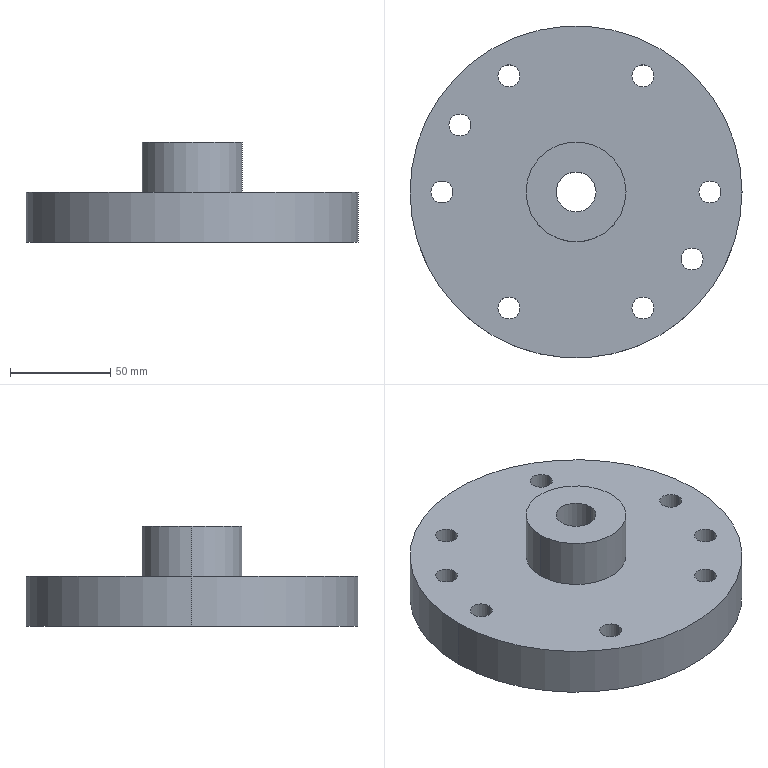Part | SolidWorks | features ICE 5, Chamfer 1, Extrusion 1 | 1 solid | 34 faces | box 166 x 166 x 50 mm | volume 495390 mm3 | cylinder 26 | plane 6 | cone 2 | commonest cylinder face diameters 11 x16 18 x4 20 x2 50 x2 166 x2
STEP:
#1=CARTESIAN_POINT('',(42.5,-58.024,12.));
#2=VERTEX_POINT('',#1);
#3=CARTESIAN_POINT('',(24.5,-58.024,12.));
#4=VERTEX_POINT('',#3);
#5=CARTESIAN_POINT('',(33.5,-58.024,12.));
#6=DIRECTION('',(0.,0.,-1.));
#7=DIRECTION('',(-1.,0.,0.));
#8=AXIS2_PLACEMENT_3D('',#5,#6,#7);
#9=CIRCLE('',#8,9.);
#10=EDGE_CURVE('',#2,#4,#9,.T.);
#11=ORIENTED_EDGE('',*,*,#10,.F.);
#12=CARTESIAN_POINT('',(42.5,-58.024,0.));
#13=VERTEX_POINT('',#12);
#14=CARTESIAN_POINT('',(42.5,-58.024,12.));
#15=DIRECTION('',(0.,0.,-1.));
#16=VECTOR('',#15,1000.);
#17=LINE('',#14,#16);
#18=EDGE_CURVE('',#2,#13,#17,.T.);
#19=ORIENTED_EDGE('',*,*,#18,.T.);
#20=CARTESIAN_POINT('',(24.5,-58.024,0.));
#21=VERTEX_POINT('',#20);
#22=CARTESIAN_POINT('',(33.5,-58.024,0.));
#23=DIRECTION('',(0.,0.,-1.));
#24=DIRECTION('',(-1.,0.,0.));
#25=AXIS2_PLACEMENT_3D('',#22,#23,#24);
#26=CIRCLE('',#25,9.);
#27=EDGE_CURVE('',#13,#21,#26,.T.);
#28=ORIENTED_EDGE('',*,*,#27,.T.);
#29=CARTESIAN_POINT('',(24.5,-58.024,12.));
#30=DIRECTION('',(0.,0.,-1.));
#31=VECTOR('',#30,1000.);
#32=LINE('',#29,#31);
#33=EDGE_CURVE('',#4,#21,#32,.T.);
#34=ORIENTED_EDGE('',*,*,#33,.F.);
#35=EDGE_LOOP('',(#11,#19,#28,#34));
#36=FACE_OUTER_BOUND('',#35,.T.);
#37=CARTESIAN_POINT('',(33.5,-58.024,12.));
#38=DIRECTION('',(0.,0.,-1.));
#39=DIRECTION('',(-1.,0.,0.));
#40=AXIS2_PLACEMENT_3D('',#37,#38,#39);
#41=CYLINDRICAL_SURFACE('',#40,9.);
#42=ADVANCED_FACE('',(#36),#41,.F.);
#43=CARTESIAN_POINT('',(-24.5,58.024,12.));
#44=VERTEX_POINT('',#43);
#45=CARTESIAN_POINT('',(-42.5,58.024,12.));
#46=VERTEX_POINT('',#45);
#47=CARTESIAN_POINT('',(-33.5,58.024,12.));
#48=DIRECTION('',(0.,0.,-1.));
#49=DIRECTION('',(-1.,0.,0.));
#50=AXIS2_PLACEMENT_3D('',#47,#48,#49);
#51=CIRCLE('',#50,9.);
#52=EDGE_CURVE('',#44,#46,#51,.T.);
#53=ORIENTED_EDGE('',*,*,#52,.F.);
#54=CARTESIAN_POINT('',(-24.5,58.024,0.));
#55=VERTEX_POINT('',#54);
#56=CARTESIAN_POINT('',(-24.5,58.024,12.));
#57=DIRECTION('',(0.,0.,-1.));
#58=VECTOR('',#57,1000.);
#59=LINE('',#56,#58);
#60=EDGE_CURVE('',#44,#55,#59,.T.);
#61=ORIENTED_EDGE('',*,*,#60,.T.);
#62=CARTESIAN_POINT('',(-42.5,58.024,0.));
#63=VERTEX_POINT('',#62);
#64=CARTESIAN_POINT('',(-33.5,58.024,0.));
#65=DIRECTION('',(0.,0.,-1.));
#66=DIRECTION('',(-1.,0.,0.));
#67=AXIS2_PLACEMENT_3D('',#64,#65,#66);
#68=CIRCLE('',#67,9.);
#69=EDGE_CURVE('',#55,#63,#68,.T.);
#70=ORIENTED_EDGE('',*,*,#69,.T.);
#71=CARTESIAN_POINT('',(-42.5,58.024,12.));
#72=DIRECTION('',(0.,0.,-1.));
#73=VECTOR('',#72,1000.);
#74=LINE('',#71,#73);
#75=EDGE_CURVE('',#46,#63,#74,.T.);
#76=ORIENTED_EDGE('',*,*,#75,.F.);
#77=EDGE_LOOP('',(#53,#61,#70,#76));
#78=FACE_OUTER_BOUND('',#77,.T.);
#79=CARTESIAN_POINT('',(-33.5,58.024,12.));
#80=DIRECTION('',(0.,0.,-1.));
#81=DIRECTION('',(-1.,0.,0.));
#82=AXIS2_PLACEMENT_3D('',#79,#80,#81);
#83=CYLINDRICAL_SURFACE('',#82,9.);
#84=ADVANCED_FACE('',(#78),#83,.F.);
#85=CARTESIAN_POINT('',(10.,0.,50.));
#86=VERTEX_POINT('',#85);
#87=CARTESIAN_POINT('',(-10.,0.,50.));
#88=VERTEX_POINT('',#87);
#89=CARTESIAN_POINT('',(0.,0.,50.));
#90=DIRECTION('',(0.,0.,-1.));
#91=DIRECTION('',(-1.,0.,0.));
#92=AXIS2_PLACEMENT_3D('',#89,#90,#91);
#93=CIRCLE('',#92,10.);
#94=EDGE_CURVE('',#86,#88,#93,.T.);
#95=ORIENTED_EDGE('',*,*,#94,.F.);
#96=CARTESIAN_POINT('',(10.,0.,7.));
#97=VERTEX_POINT('',#96);
#98=CARTESIAN_POINT('',(10.,0.,50.));
#99=DIRECTION('',(0.,0.,-1.));
#100=VECTOR('',#99,1000.);
#101=LINE('',#98,#100);
#102=EDGE_CURVE('',#86,#97,#101,.T.);
#103=ORIENTED_EDGE('',*,*,#102,.T.);
#104=CARTESIAN_POINT('',(-10.,0.,7.));
#105=VERTEX_POINT('',#104);
#106=CARTESIAN_POINT('',(0.,0.,7.));
#107=DIRECTION('',(0.,0.,-1.));
#108=DIRECTION('',(-1.,0.,0.));
#109=AXIS2_PLACEMENT_3D('',#106,#107,#108);
#110=CIRCLE('',#109,10.);
#111=EDGE_CURVE('',#97,#105,#110,.T.);
#112=ORIENTED_EDGE('',*,*,#111,.T.);
#113=CARTESIAN_POINT('',(-10.,0.,50.));
#114=DIRECTION('',(0.,0.,-1.));
#115=VECTOR('',#114,1000.);
#116=LINE('',#113,#115);
#117=EDGE_CURVE('',#88,#105,#116,.T.);
#118=ORIENTED_EDGE('',*,*,#117,.F.);
#119=EDGE_LOOP('',(#95,#103,#112,#118));
#120=FACE_OUTER_BOUND('',#119,.T.);
#121=CARTESIAN_POINT('',(0.,0.,50.));
#122=DIRECTION('',(0.,0.,-1.));
#123=DIRECTION('',(-1.,0.,0.));
#124=AXIS2_PLACEMENT_3D('',#121,#122,#123);
#125=CYLINDRICAL_SURFACE('',#124,10.);
#126=ADVANCED_FACE('',(#120),#125,.F.);
#127=CARTESIAN_POINT('',(-63.524,33.5,25.));
#128=VERTEX_POINT('',#127);
#129=CARTESIAN_POINT('',(-52.524,33.5,25.));
#130=VERTEX_POINT('',#129);
#131=CARTESIAN_POINT('',(-58.024,33.5,25.));
#132=DIRECTION('',(0.,0.,1.));
#133=DIRECTION('',(1.,0.,0.));
#134=AXIS2_PLACEMENT_3D('',#131,#132,#133);
#135=CIRCLE('',#134,5.5);
#136=EDGE_CURVE('',#128,#130,#135,.T.);
#137=ORIENTED_EDGE('',*,*,#136,.T.);
#138=CARTESIAN_POINT('',(-52.524,33.5,0.));
#139=VERTEX_POINT('',#138);
#140=CARTESIAN_POINT('',(-52.524,33.5,50.));
#141=DIRECTION('',(0.,0.,-1.));
#142=VECTOR('',#141,1000.);
#143=LINE('',#140,#142);
#144=EDGE_CURVE('',#130,#139,#143,.T.);
#145=ORIENTED_EDGE('',*,*,#144,.T.);
#146=CARTESIAN_POINT('',(-63.524,33.5,0.));
#147=VERTEX_POINT('',#146);
#148=CARTESIAN_POINT('',(-58.024,33.5,0.));
#149=DIRECTION('',(0.,0.,-1.));
#150=DIRECTION('',(-1.,0.,0.));
#151=AXIS2_PLACEMENT_3D('',#148,#149,#150);
#152=CIRCLE('',#151,5.5);
#153=EDGE_CURVE('',#139,#147,#152,.T.);
#154=ORIENTED_EDGE('',*,*,#153,.T.);
#155=CARTESIAN_POINT('',(-63.524,33.5,50.));
#156=DIRECTION('',(0.,0.,-1.));
#157=VECTOR('',#156,1000.);
#158=LINE('',#155,#157);
#159=EDGE_CURVE('',#128,#147,#158,.T.);
#160=ORIENTED_EDGE('',*,*,#159,.F.);
#161=EDGE_LOOP('',(#137,#145,#154,#160));
#162=FACE_OUTER_BOUND('',#161,.T.);
#163=CARTESIAN_POINT('',(-58.024,33.5,50.));
#164=DIRECTION('',(0.,0.,-1.));
#165=DIRECTION('',(-1.,0.,0.));
#166=AXIS2_PLACEMENT_3D('',#163,#164,#165);
#167=CYLINDRICAL_SURFACE('',#166,5.5);
#168=ADVANCED_FACE('',(#162),#167,.F.);
#169=CARTESIAN_POINT('',(-39.,-58.024,25.));
#170=VERTEX_POINT('',#169);
#171=CARTESIAN_POINT('',(-28.,-58.024,25.));
#172=VERTEX_POINT('',#171);
#173=CARTESIAN_POINT('',(-33.5,-58.024,25.));
#174=DIRECTION('',(0.,0.,1.));
#175=DIRECTION('',(1.,0.,0.));
#176=AXIS2_PLACEMENT_3D('',#173,#174,#175);
#177=CIRCLE('',#176,5.5);
#178=EDGE_CURVE('',#170,#172,#177,.T.);
#179=ORIENTED_EDGE('',*,*,#178,.T.);
#180=CARTESIAN_POINT('',(-28.,-58.024,0.));
#181=VERTEX_POINT('',#180);
#182=CARTESIAN_POINT('',(-28.,-58.024,50.));
#183=DIRECTION('',(0.,0.,-1.));
#184=VECTOR('',#183,1000.);
#185=LINE('',#182,#184);
#186=EDGE_CURVE('',#172,#181,#185,.T.);
#187=ORIENTED_EDGE('',*,*,#186,.T.);
#188=CARTESIAN_POINT('',(-39.,-58.024,0.));
#189=VERTEX_POINT('',#188);
#190=CARTESIAN_POINT('',(-33.5,-58.024,0.));
#191=DIRECTION('',(0.,0.,-1.));
#192=DIRECTION('',(-1.,0.,0.));
#193=AXIS2_PLACEMENT_3D('',#190,#191,#192);
#194=CIRCLE('',#193,5.5);
#195=EDGE_CURVE('',#181,#189,#194,.T.);
#196=ORIENTED_EDGE('',*,*,#195,.T.);
#197=CARTESIAN_POINT('',(-39.,-58.024,50.));
#198=DIRECTION('',(0.,0.,-1.));
#199=VECTOR('',#198,1000.);
#200=LINE('',#197,#199);
#201=EDGE_CURVE('',#170,#189,#200,.T.);
#202=ORIENTED_EDGE('',*,*,#201,.F.);
#203=EDGE_LOOP('',(#179,#187,#196,#202));
#204=FACE_OUTER_BOUND('',#203,.T.);
#205=CARTESIAN_POINT('',(-33.5,-58.024,50.));
#206=DIRECTION('',(0.,0.,-1.));
#207=DIRECTION('',(-1.,0.,0.));
#208=AXIS2_PLACEMENT_3D('',#205,#206,#207);
#209=CYLINDRICAL_SURFACE('',#208,5.5);
#210=ADVANCED_FACE('',(#204),#209,.F.);
#211=CARTESIAN_POINT('',(52.524,-33.5,25.));
#212=VERTEX_POINT('',#211);
#213=CARTESIAN_POINT('',(63.524,-33.5,25.));
#214=VERTEX_POINT('',#213);
#215=CARTESIAN_POINT('',(58.024,-33.5,25.));
#216=DIRECTION('',(0.,0.,1.));
#217=DIRECTION('',(1.,0.,0.));
#218=AXIS2_PLACEMENT_3D('',#215,#216,#217);
#219=CIRCLE('',#218,5.5);
#220=EDGE_CURVE('',#212,#214,#219,.T.);
#221=ORIENTED_EDGE('',*,*,#220,.T.);
#222=CARTESIAN_POINT('',(63.524,-33.5,0.));
#223=VERTEX_POINT('',#222);
#224=CARTESIAN_POINT('',(63.524,-33.5,50.));
#225=DIRECTION('',(0.,0.,-1.));
#226=VECTOR('',#225,1000.);
#227=LINE('',#224,#226);
#228=EDGE_CURVE('',#214,#223,#227,.T.);
#229=ORIENTED_EDGE('',*,*,#228,.T.);
#230=CARTESIAN_POINT('',(52.524,-33.5,0.));
#231=VERTEX_POINT('',#230);
#232=CARTESIAN_POINT('',(58.024,-33.5,0.));
#233=DIRECTION('',(0.,0.,-1.));
#234=DIRECTION('',(-1.,0.,0.));
#235=AXIS2_PLACEMENT_3D('',#232,#233,#234);
#236=CIRCLE('',#235,5.5);
#237=EDGE_CURVE('',#223,#231,#236,.T.);
#238=ORIENTED_EDGE('',*,*,#237,.T.);
#239=CARTESIAN_POINT('',(52.524,-33.5,50.));
#240=DIRECTION('',(0.,0.,-1.));
#241=VECTOR('',#240,1000.);
#242=LINE('',#239,#241);
#243=EDGE_CURVE('',#212,#231,#242,.T.);
#244=ORIENTED_EDGE('',*,*,#243,.F.);
#245=EDGE_LOOP('',(#221,#229,#238,#244));
#246=FACE_OUTER_BOUND('',#245,.T.);
#247=CARTESIAN_POINT('',(58.024,-33.5,50.));
#248=DIRECTION('',(0.,0.,-1.));
#249=DIRECTION('',(-1.,0.,0.));
#250=AXIS2_PLACEMENT_3D('',#247,#248,#249);
#251=CYLINDRICAL_SURFACE('',#250,5.5);
#252=ADVANCED_FACE('',(#246),#251,.F.);
#253=CARTESIAN_POINT('',(61.5,0.,25.));
#254=VERTEX_POINT('',#253);
#255=CARTESIAN_POINT('',(72.5,0.,25.));
#256=VERTEX_POINT('',#255);
#257=CARTESIAN_POINT('',(67.,0.,25.));
#258=DIRECTION('',(0.,0.,1.));
#259=DIRECTION('',(1.,0.,0.));
#260=AXIS2_PLACEMENT_3D('',#257,#258,#259);
#261=CIRCLE('',#260,5.5);
#262=EDGE_CURVE('',#254,#256,#261,.T.);
#263=ORIENTED_EDGE('',*,*,#262,.T.);
#264=CARTESIAN_POINT('',(72.5,0.,0.));
#265=VERTEX_POINT('',#264);
#266=CARTESIAN_POINT('',(72.5,0.,50.));
#267=DIRECTION('',(0.,0.,-1.));
#268=VECTOR('',#267,1000.);
#269=LINE('',#266,#268);
#270=EDGE_CURVE('',#256,#265,#269,.T.);
#271=ORIENTED_EDGE('',*,*,#270,.T.);
#272=CARTESIAN_POINT('',(61.5,0.,0.));
#273=VERTEX_POINT('',#272);
#274=CARTESIAN_POINT('',(67.,0.,0.));
#275=DIRECTION('',(0.,0.,-1.));
#276=DIRECTION('',(-1.,0.,0.));
#277=AXIS2_PLACEMENT_3D('',#274,#275,#276);
#278=CIRCLE('',#277,5.5);
#279=EDGE_CURVE('',#265,#273,#278,.T.);
#280=ORIENTED_EDGE('',*,*,#279,.T.);
#281=CARTESIAN_POINT('',(61.5,0.,50.));
#282=DIRECTION('',(0.,0.,-1.));
#283=VECTOR('',#282,1000.);
#284=LINE('',#281,#283);
#285=EDGE_CURVE('',#254,#273,#284,.T.);
#286=ORIENTED_EDGE('',*,*,#285,.F.);
#287=EDGE_LOOP('',(#263,#271,#280,#286));
#288=FACE_OUTER_BOUND('',#287,.T.);
#289=CARTESIAN_POINT('',(67.,0.,50.));
#290=DIRECTION('',(0.,0.,-1.));
#291=DIRECTION('',(-1.,0.,0.));
#292=AXIS2_PLACEMENT_3D('',#289,#290,#291);
#293=CYLINDRICAL_SURFACE('',#292,5.5);
#294=ADVANCED_FACE('',(#288),#293,.F.);
#295=CARTESIAN_POINT('',(28.,58.024,25.));
#296=VERTEX_POINT('',#295);
#297=CARTESIAN_POINT('',(39.,58.024,25.));
#298=VERTEX_POINT('',#297);
#299=CARTESIAN_POINT('',(33.5,58.024,25.));
#300=DIRECTION('',(0.,0.,1.));
#301=DIRECTION('',(1.,0.,0.));
#302=AXIS2_PLACEMENT_3D('',#299,#300,#301);
#303=CIRCLE('',#302,5.5);
#304=EDGE_CURVE('',#296,#298,#303,.T.);
#305=ORIENTED_EDGE('',*,*,#304,.T.);
#306=CARTESIAN_POINT('',(39.,58.024,0.));
#307=VERTEX_POINT('',#306);
#308=CARTESIAN_POINT('',(39.,58.024,50.));
#309=DIRECTION('',(0.,0.,-1.));
#310=VECTOR('',#309,1000.);
#311=LINE('',#308,#310);
#312=EDGE_CURVE('',#298,#307,#311,.T.);
#313=ORIENTED_EDGE('',*,*,#312,.T.);
#314=CARTESIAN_POINT('',(28.,58.024,0.));
#315=VERTEX_POINT('',#314);
#316=CARTESIAN_POINT('',(33.5,58.024,0.));
#317=DIRECTION('',(0.,0.,-1.));
#318=DIRECTION('',(-1.,0.,0.));
#319=AXIS2_PLACEMENT_3D('',#316,#317,#318);
#320=CIRCLE('',#319,5.5);
#321=EDGE_CURVE('',#307,#315,#320,.T.);
#322=ORIENTED_EDGE('',*,*,#321,.T.);
#323=CARTESIAN_POINT('',(28.,58.024,50.));
#324=DIRECTION('',(0.,0.,-1.));
#325=VECTOR('',#324,1000.);
#326=LINE('',#323,#325);
#327=EDGE_CURVE('',#296,#315,#326,.T.);
#328=ORIENTED_EDGE('',*,*,#327,.F.);
#329=EDGE_LOOP('',(#305,#313,#322,#328));
#330=FACE_OUTER_BOUND('',#329,.T.);
#331=CARTESIAN_POINT('',(33.5,58.024,50.));
#332=DIRECTION('',(0.,0.,-1.));
#333=DIRECTION('',(-1.,0.,0.));
#334=AXIS2_PLACEMENT_3D('',#331,#332,#333);
#335=CYLINDRICAL_SURFACE('',#334,5.5);
#336=ADVANCED_FACE('',(#330),#335,.F.);
#337=CARTESIAN_POINT('',(-72.5,0.,25.));
#338=VERTEX_POINT('',#337);
#339=CARTESIAN_POINT('',(-61.5,0.,25.));
#340=VERTEX_POINT('',#339);
#341=CARTESIAN_POINT('',(-67.,0.,25.));
#342=DIRECTION('',(0.,0.,1.));
#343=DIRECTION('',(1.,0.,0.));
#344=AXIS2_PLACEMENT_3D('',#341,#342,#343);
#345=CIRCLE('',#344,5.5);
#346=EDGE_CURVE('',#338,#340,#345,.T.);
#347=ORIENTED_EDGE('',*,*,#346,.T.);
#348=CARTESIAN_POINT('',(-61.5,0.,0.));
#349=VERTEX_POINT('',#348);
#350=CARTESIAN_POINT('',(-61.5,0.,50.));
#351=DIRECTION('',(0.,0.,-1.));
#352=VECTOR('',#351,1000.);
#353=LINE('',#350,#352);
#354=EDGE_CURVE('',#340,#349,#353,.T.);
#355=ORIENTED_EDGE('',*,*,#354,.T.);
#356=CARTESIAN_POINT('',(-72.5,0.,0.));
#357=VERTEX_POINT('',#356);
#358=CARTESIAN_POINT('',(-67.,0.,0.));
#359=DIRECTION('',(0.,0.,-1.));
#360=DIRECTION('',(-1.,0.,0.));
#361=AXIS2_PLACEMENT_3D('',#358,#359,#360);
#362=CIRCLE('',#361,5.5);
#363=EDGE_CURVE('',#349,#357,#362,.T.);
#364=ORIENTED_EDGE('',*,*,#363,.T.);
#365=CARTESIAN_POINT('',(-72.5,0.,50.));
#366=DIRECTION('',(0.,0.,-1.));
#367=VECTOR('',#366,1000.);
#368=LINE('',#365,#367);
#369=EDGE_CURVE('',#338,#357,#368,.T.);
#370=ORIENTED_EDGE('',*,*,#369,.F.);
#371=EDGE_LOOP('',(#347,#355,#364,#370));
#372=FACE_OUTER_BOUND('',#371,.T.);
#373=CARTESIAN_POINT('',(-67.,0.,50.));
#374=DIRECTION('',(0.,0.,-1.));
#375=DIRECTION('',(-1.,0.,0.));
#376=AXIS2_PLACEMENT_3D('',#373,#374,#375);
#377=CYLINDRICAL_SURFACE('',#376,5.5);
#378=ADVANCED_FACE('',(#372),#377,.F.);
#379=CARTESIAN_POINT('',(48.,0.,7.));
#380=VERTEX_POINT('',#379);
#381=CARTESIAN_POINT('',(-48.,0.,7.));
#382=VERTEX_POINT('',#381);
#383=CARTESIAN_POINT('',(0.,0.,7.));
#384=DIRECTION('',(0.,0.,-1.));
#385=DIRECTION('',(-1.,0.,0.));
#386=AXIS2_PLACEMENT_3D('',#383,#384,#385);
#387=CIRCLE('',#386,48.);
#388=EDGE_CURVE('',#380,#382,#387,.T.);
#389=ORIENTED_EDGE('',*,*,#388,.F.);
#390=CARTESIAN_POINT('',(55.,0.,0.));
#391=VERTEX_POINT('',#390);
#392=CARTESIAN_POINT('',(48.,0.,7.));
#393=DIRECTION('',(0.7071,0.,-0.7071));
#394=VECTOR('',#393,1000.);
#395=LINE('',#392,#394);
#396=EDGE_CURVE('',#380,#391,#395,.T.);
#397=ORIENTED_EDGE('',*,*,#396,.T.);
#398=CARTESIAN_POINT('',(-55.,0.,0.));
#399=VERTEX_POINT('',#398);
#400=CARTESIAN_POINT('',(0.,0.,0.));
#401=DIRECTION('',(0.,0.,-1.));
#402=DIRECTION('',(-1.,0.,0.));
#403=AXIS2_PLACEMENT_3D('',#400,#401,#402);
#404=CIRCLE('',#403,55.);
#405=EDGE_CURVE('',#391,#399,#404,.T.);
#406=ORIENTED_EDGE('',*,*,#405,.T.);
#407=CARTESIAN_POINT('',(-48.,0.,7.));
#408=DIRECTION('',(-0.7071,0.,-0.7071));
#409=VECTOR('',#408,1000.);
#410=LINE('',#407,#409);
#411=EDGE_CURVE('',#382,#399,#410,.T.);
#412=ORIENTED_EDGE('',*,*,#411,.F.);
#413=EDGE_LOOP('',(#389,#397,#406,#412));
#414=FACE_OUTER_BOUND('',#413,.T.);
#415=CARTESIAN_POINT('',(0.,0.,7.));
#416=DIRECTION('',(0.,0.,-1.));
#417=DIRECTION('',(-1.,0.,0.));
#418=AXIS2_PLACEMENT_3D('',#415,#416,#417);
#419=CONICAL_SURFACE('',#418,48.,0.7854);
#420=ADVANCED_FACE('',(#414),#419,.F.);
#421=CARTESIAN_POINT('',(25.,0.,50.));
#422=VERTEX_POINT('',#421);
#423=CARTESIAN_POINT('',(-25.,0.,50.));
#424=VERTEX_POINT('',#423);
#425=CARTESIAN_POINT('',(0.,0.,50.));
#426=DIRECTION('',(0.,0.,1.));
#427=DIRECTION('',(1.,0.,0.));
#428=AXIS2_PLACEMENT_3D('',#425,#426,#427);
#429=CIRCLE('',#428,25.);
#430=EDGE_CURVE('',#422,#424,#429,.T.);
#431=ORIENTED_EDGE('',*,*,#430,.F.);
#432=CARTESIAN_POINT('',(25.,0.,25.));
#433=VERTEX_POINT('',#432);
#434=CARTESIAN_POINT('',(25.,0.,50.));
#435=DIRECTION('',(0.,0.,-1.));
#436=VECTOR('',#435,1000.);
#437=LINE('',#434,#436);
#438=EDGE_CURVE('',#422,#433,#437,.T.);
#439=ORIENTED_EDGE('',*,*,#438,.T.);
#440=CARTESIAN_POINT('',(-25.,0.,25.));
#441=VERTEX_POINT('',#440);
#442=CARTESIAN_POINT('',(0.,0.,25.));
#443=DIRECTION('',(0.,0.,1.));
#444=DIRECTION('',(1.,0.,0.));
#445=AXIS2_PLACEMENT_3D('',#442,#443,#444);
#446=CIRCLE('',#445,25.);
#447=EDGE_CURVE('',#433,#441,#446,.T.);
#448=ORIENTED_EDGE('',*,*,#447,.T.);
#449=CARTESIAN_POINT('',(-25.,0.,50.));
#450=DIRECTION('',(0.,0.,-1.));
#451=VECTOR('',#450,1000.);
#452=LINE('',#449,#451);
#453=EDGE_CURVE('',#424,#441,#452,.T.);
#454=ORIENTED_EDGE('',*,*,#453,.F.);
#455=EDGE_LOOP('',(#431,#439,#448,#454));
#456=FACE_OUTER_BOUND('',#455,.T.);
#457=CARTESIAN_POINT('',(0.,0.,50.));
#458=DIRECTION('',(0.,0.,-1.));
#459=DIRECTION('',(-1.,0.,0.));
#460=AXIS2_PLACEMENT_3D('',#457,#458,#459);
#461=CYLINDRICAL_SURFACE('',#460,25.);
#462=ADVANCED_FACE('',(#456),#461,.T.);
#463=CARTESIAN_POINT('',(83.,0.,25.));
#464=VERTEX_POINT('',#463);
#465=CARTESIAN_POINT('',(-83.,0.,25.));
#466=VERTEX_POINT('',#465);
#467=CARTESIAN_POINT('',(0.,0.,25.));
#468=DIRECTION('',(0.,0.,1.));
#469=DIRECTION('',(1.,0.,0.));
#470=AXIS2_PLACEMENT_3D('',#467,#468,#469);
#471=CIRCLE('',#470,83.);
#472=EDGE_CURVE('',#464,#466,#471,.T.);
#473=ORIENTED_EDGE('',*,*,#472,.F.);
#474=CARTESIAN_POINT('',(83.,0.,0.));
#475=VERTEX_POINT('',#474);
#476=CARTESIAN_POINT('',(83.,0.,25.));
#477=DIRECTION('',(0.,0.,-1.));
#478=VECTOR('',#477,1000.);
#479=LINE('',#476,#478);
#480=EDGE_CURVE('',#464,#475,#479,.T.);
#481=ORIENTED_EDGE('',*,*,#480,.T.);
#482=CARTESIAN_POINT('',(-83.,0.,0.));
#483=VERTEX_POINT('',#482);
#484=CARTESIAN_POINT('',(0.,0.,0.));
#485=DIRECTION('',(0.,0.,1.));
#486=DIRECTION('',(1.,0.,0.));
#487=AXIS2_PLACEMENT_3D('',#484,#485,#486);
#488=CIRCLE('',#487,83.);
#489=EDGE_CURVE('',#475,#483,#488,.T.);
#490=ORIENTED_EDGE('',*,*,#489,.T.);
#491=CARTESIAN_POINT('',(-83.,0.,25.));
#492=DIRECTION('',(0.,0.,-1.));
#493=VECTOR('',#492,1000.);
#494=LINE('',#491,#493);
#495=EDGE_CURVE('',#466,#483,#494,.T.);
#496=ORIENTED_EDGE('',*,*,#495,.F.);
#497=EDGE_LOOP('',(#473,#481,#490,#496));
#498=FACE_OUTER_BOUND('',#497,.T.);
#499=CARTESIAN_POINT('',(0.,0.,25.));
#500=DIRECTION('',(0.,0.,-1.));
#501=DIRECTION('',(-1.,0.,0.));
#502=AXIS2_PLACEMENT_3D('',#499,#500,#501);
#503=CYLINDRICAL_SURFACE('',#502,83.);
#504=ADVANCED_FACE('',(#498),#503,.T.);
#505=CARTESIAN_POINT('',(-39.,58.024,25.));
#506=VERTEX_POINT('',#505);
#507=CARTESIAN_POINT('',(-28.,58.024,25.));
#508=VERTEX_POINT('',#507);
#509=CARTESIAN_POINT('',(-33.5,58.024,25.));
#510=DIRECTION('',(0.,0.,1.));
#511=DIRECTION('',(1.,0.,0.));
#512=AXIS2_PLACEMENT_3D('',#509,#510,#511);
#513=CIRCLE('',#512,5.5);
#514=EDGE_CURVE('',#506,#508,#513,.T.);
#515=ORIENTED_EDGE('',*,*,#514,.T.);
#516=CARTESIAN_POINT('',(-28.,58.024,12.));
#517=VERTEX_POINT('',#516);
#518=CARTESIAN_POINT('',(-28.,58.024,50.));
#519=DIRECTION('',(0.,0.,-1.));
#520=VECTOR('',#519,1000.);
#521=LINE('',#518,#520);
#522=EDGE_CURVE('',#508,#517,#521,.T.);
#523=ORIENTED_EDGE('',*,*,#522,.T.);
#524=CARTESIAN_POINT('',(-39.,58.024,12.));
#525=VERTEX_POINT('',#524);
#526=CARTESIAN_POINT('',(-33.5,58.024,12.));
#527=DIRECTION('',(0.,0.,1.));
#528=DIRECTION('',(-1.,0.,0.));
#529=AXIS2_PLACEMENT_3D('',#526,#527,#528);
#530=CIRCLE('',#529,5.5);
#531=EDGE_CURVE('',#525,#517,#530,.T.);
#532=ORIENTED_EDGE('',*,*,#531,.F.);
#533=CARTESIAN_POINT('',(-39.,58.024,50.));
#534=DIRECTION('',(0.,0.,-1.));
#535=VECTOR('',#534,1000.);
#536=LINE('',#533,#535);
#537=EDGE_CURVE('',#506,#525,#536,.T.);
#538=ORIENTED_EDGE('',*,*,#537,.F.);
#539=EDGE_LOOP('',(#515,#523,#532,#538));
#540=FACE_OUTER_BOUND('',#539,.T.);
#541=CARTESIAN_POINT('',(-33.5,58.024,50.));
#542=DIRECTION('',(0.,0.,-1.));
#543=DIRECTION('',(-1.,0.,0.));
#544=AXIS2_PLACEMENT_3D('',#541,#542,#543);
#545=CYLINDRICAL_SURFACE('',#544,5.5);
#546=ADVANCED_FACE('',(#540),#545,.F.);
#547=CARTESIAN_POINT('',(28.,-58.024,25.));
#548=VERTEX_POINT('',#547);
#549=CARTESIAN_POINT('',(39.,-58.024,25.));
#550=VERTEX_POINT('',#549);
#551=CARTESIAN_POINT('',(33.5,-58.024,25.));
#552=DIRECTION('',(0.,0.,1.));
#553=DIRECTION('',(1.,0.,0.));
#554=AXIS2_PLACEMENT_3D('',#551,#552,#553);
#555=CIRCLE('',#554,5.5);
#556=EDGE_CURVE('',#548,#550,#555,.T.);
#557=ORIENTED_EDGE('',*,*,#556,.T.);
#558=CARTESIAN_POINT('',(39.,-58.024,12.));
#559=VERTEX_POINT('',#558);
#560=CARTESIAN_POINT('',(39.,-58.024,50.));
#561=DIRECTION('',(0.,0.,-1.));
#562=VECTOR('',#561,1000.);
#563=LINE('',#560,#562);
#564=EDGE_CURVE('',#550,#559,#563,.T.);
#565=ORIENTED_EDGE('',*,*,#564,.T.);
#566=CARTESIAN_POINT('',(28.,-58.024,12.));
#567=VERTEX_POINT('',#566);
#568=CARTESIAN_POINT('',(33.5,-58.024,12.));
#569=DIRECTION('',(0.,0.,1.));
#570=DIRECTION('',(-1.,0.,0.));
#571=AXIS2_PLACEMENT_3D('',#568,#569,#570);
#572=CIRCLE('',#571,5.5);
#573=EDGE_CURVE('',#567,#559,#572,.T.);
#574=ORIENTED_EDGE('',*,*,#573,.F.);
#575=CARTESIAN_POINT('',(28.,-58.024,50.));
#576=DIRECTION('',(0.,0.,-1.));
#577=VECTOR('',#576,1000.);
#578=LINE('',#575,#577);
#579=EDGE_CURVE('',#548,#567,#578,.T.);
#580=ORIENTED_EDGE('',*,*,#579,.F.);
#581=EDGE_LOOP('',(#557,#565,#574,#580));
#582=FACE_OUTER_BOUND('',#581,.T.);
#583=CARTESIAN_POINT('',(33.5,-58.024,50.));
#584=DIRECTION('',(0.,0.,-1.));
#585=DIRECTION('',(-1.,0.,0.));
#586=AXIS2_PLACEMENT_3D('',#583,#584,#585);
#587=CYLINDRICAL_SURFACE('',#586,5.5);
#588=ADVANCED_FACE('',(#582),#587,.F.);
#589=ORIENTED_EDGE('',*,*,#564,.F.);
#590=CARTESIAN_POINT('',(33.5,-58.024,25.));
#591=DIRECTION('',(0.,0.,1.));
#592=DIRECTION('',(1.,0.,0.));
#593=AXIS2_PLACEMENT_3D('',#590,#591,#592);
#594=CIRCLE('',#593,5.5);
#595=EDGE_CURVE('',#550,#548,#594,.T.);
#596=ORIENTED_EDGE('',*,*,#595,.T.);
#597=ORIENTED_EDGE('',*,*,#579,.T.);
#598=CARTESIAN_POINT('',(33.5,-58.024,12.));
#599=DIRECTION('',(0.,0.,1.));
#600=DIRECTION('',(-1.,0.,0.));
#601=AXIS2_PLACEMENT_3D('',#598,#599,#600);
#602=CIRCLE('',#601,5.5);
#603=EDGE_CURVE('',#559,#567,#602,.T.);
#604=ORIENTED_EDGE('',*,*,#603,.F.);
#605=EDGE_LOOP('',(#589,#596,#597,#604));
#606=FACE_OUTER_BOUND('',#605,.T.);
#607=CARTESIAN_POINT('',(33.5,-58.024,50.));
#608=DIRECTION('',(0.,0.,-1.));
#609=DIRECTION('',(-1.,0.,0.));
#610=AXIS2_PLACEMENT_3D('',#607,#608,#609);
#611=CYLINDRICAL_SURFACE('',#610,5.5);
#612=ADVANCED_FACE('',(#606),#611,.F.);
#613=ORIENTED_EDGE('',*,*,#522,.F.);
#614=CARTESIAN_POINT('',(-33.5,58.024,25.));
#615=DIRECTION('',(0.,0.,1.));
#616=DIRECTION('',(1.,0.,0.));
#617=AXIS2_PLACEMENT_3D('',#614,#615,#616);
#618=CIRCLE('',#617,5.5);
#619=EDGE_CURVE('',#508,#506,#618,.T.);
#620=ORIENTED_EDGE('',*,*,#619,.T.);
#621=ORIENTED_EDGE('',*,*,#537,.T.);
#622=CARTESIAN_POINT('',(-33.5,58.024,12.));
#623=DIRECTION('',(0.,0.,1.));
#624=DIRECTION('',(-1.,0.,0.));
#625=AXIS2_PLACEMENT_3D('',#622,#623,#624);
#626=CIRCLE('',#625,5.5);
#627=EDGE_CURVE('',#517,#525,#626,.T.);
#628=ORIENTED_EDGE('',*,*,#627,.F.);
#629=EDGE_LOOP('',(#613,#620,#621,#628));
#630=FACE_OUTER_BOUND('',#629,.T.);
#631=CARTESIAN_POINT('',(-33.5,58.024,50.));
#632=DIRECTION('',(0.,0.,-1.));
#633=DIRECTION('',(-1.,0.,0.));
#634=AXIS2_PLACEMENT_3D('',#631,#632,#633);
#635=CYLINDRICAL_SURFACE('',#634,5.5);
#636=ADVANCED_FACE('',(#630),#635,.F.);
#637=ORIENTED_EDGE('',*,*,#136,.F.);
#638=CARTESIAN_POINT('',(-58.024,33.5,25.));
#639=DIRECTION('',(0.,0.,1.));
#640=DIRECTION('',(1.,0.,0.));
#641=AXIS2_PLACEMENT_3D('',#638,#639,#640);
#642=CIRCLE('',#641,5.5);
#643=EDGE_CURVE('',#130,#128,#642,.T.);
#644=ORIENTED_EDGE('',*,*,#643,.F.);
#645=EDGE_LOOP('',(#637,#644));
#646=FACE_BOUND('',#645,.T.);
#647=ORIENTED_EDGE('',*,*,#514,.F.);
#648=ORIENTED_EDGE('',*,*,#619,.F.);
#649=EDGE_LOOP('',(#647,#648));
#650=FACE_BOUND('',#649,.T.);
#651=ORIENTED_EDGE('',*,*,#178,.F.);
#652=CARTESIAN_POINT('',(-33.5,-58.024,25.));
#653=DIRECTION('',(0.,0.,1.));
#654=DIRECTION('',(1.,0.,0.));
#655=AXIS2_PLACEMENT_3D('',#652,#653,#654);
#656=CIRCLE('',#655,5.5);
#657=EDGE_CURVE('',#172,#170,#656,.T.);
#658=ORIENTED_EDGE('',*,*,#657,.F.);
#659=EDGE_LOOP('',(#651,#658));
#660=FACE_BOUND('',#659,.T.);
#661=ORIENTED_EDGE('',*,*,#556,.F.);
#662=ORIENTED_EDGE('',*,*,#595,.F.);
#663=EDGE_LOOP('',(#661,#662));
#664=FACE_BOUND('',#663,.T.);
#665=ORIENTED_EDGE('',*,*,#220,.F.);
#666=CARTESIAN_POINT('',(58.024,-33.5,25.));
#667=DIRECTION('',(0.,0.,1.));
#668=DIRECTION('',(1.,0.,0.));
#669=AXIS2_PLACEMENT_3D('',#666,#667,#668);
#670=CIRCLE('',#669,5.5);
#671=EDGE_CURVE('',#214,#212,#670,.T.);
#672=ORIENTED_EDGE('',*,*,#671,.F.);
#673=EDGE_LOOP('',(#665,#672));
#674=FACE_BOUND('',#673,.T.);
#675=ORIENTED_EDGE('',*,*,#262,.F.);
#676=CARTESIAN_POINT('',(67.,0.,25.));
#677=DIRECTION('',(0.,0.,1.));
#678=DIRECTION('',(1.,0.,0.));
#679=AXIS2_PLACEMENT_3D('',#676,#677,#678);
#680=CIRCLE('',#679,5.5);
#681=EDGE_CURVE('',#256,#254,#680,.T.);
#682=ORIENTED_EDGE('',*,*,#681,.F.);
#683=EDGE_LOOP('',(#675,#682));
#684=FACE_BOUND('',#683,.T.);
#685=ORIENTED_EDGE('',*,*,#304,.F.);
#686=CARTESIAN_POINT('',(33.5,58.024,25.));
#687=DIRECTION('',(0.,0.,1.));
#688=DIRECTION('',(1.,0.,0.));
#689=AXIS2_PLACEMENT_3D('',#686,#687,#688);
#690=CIRCLE('',#689,5.5);
#691=EDGE_CURVE('',#298,#296,#690,.T.);
#692=ORIENTED_EDGE('',*,*,#691,.F.);
#693=EDGE_LOOP('',(#685,#692));
#694=FACE_BOUND('',#693,.T.);
#695=ORIENTED_EDGE('',*,*,#346,.F.);
#696=CARTESIAN_POINT('',(-67.,0.,25.));
#697=DIRECTION('',(0.,0.,1.));
#698=DIRECTION('',(1.,0.,0.));
#699=AXIS2_PLACEMENT_3D('',#696,#697,#698);
#700=CIRCLE('',#699,5.5);
#701=EDGE_CURVE('',#340,#338,#700,.T.);
#702=ORIENTED_EDGE('',*,*,#701,.F.);
#703=EDGE_LOOP('',(#695,#702));
#704=FACE_BOUND('',#703,.T.);
#705=CARTESIAN_POINT('',(0.,0.,25.));
#706=DIRECTION('',(0.,0.,1.));
#707=DIRECTION('',(1.,0.,0.));
#708=AXIS2_PLACEMENT_3D('',#705,#706,#707);
#709=CIRCLE('',#708,83.);
#710=EDGE_CURVE('',#466,#464,#709,.T.);
#711=ORIENTED_EDGE('',*,*,#710,.T.);
#712=ORIENTED_EDGE('',*,*,#472,.T.);
#713=EDGE_LOOP('',(#711,#712));
#714=FACE_OUTER_BOUND('',#713,.T.);
#715=CARTESIAN_POINT('',(0.,0.,25.));
#716=DIRECTION('',(0.,0.,1.));
#717=DIRECTION('',(1.,0.,0.));
#718=AXIS2_PLACEMENT_3D('',#715,#716,#717);
#719=CIRCLE('',#718,25.);
#720=EDGE_CURVE('',#441,#433,#719,.T.);
#721=ORIENTED_EDGE('',*,*,#720,.F.);
#722=ORIENTED_EDGE('',*,*,#447,.F.);
#723=EDGE_LOOP('',(#721,#722));
#724=FACE_BOUND('',#723,.T.);
#725=CARTESIAN_POINT('',(0.,0.,25.));
#726=DIRECTION('',(0.,0.,1.));
#727=DIRECTION('',(1.,0.,0.));
#728=AXIS2_PLACEMENT_3D('',#725,#726,#727);
#729=PLANE('',#728);
#730=ADVANCED_FACE('',(#646,#650,#660,#664,#674,#684,#694,#704,#714,#724),#729,.T.);
#731=ORIENTED_EDGE('',*,*,#480,.F.);
#732=ORIENTED_EDGE('',*,*,#710,.F.);
#733=ORIENTED_EDGE('',*,*,#495,.T.);
#734=CARTESIAN_POINT('',(0.,0.,0.));
#735=DIRECTION('',(0.,0.,1.));
#736=DIRECTION('',(1.,0.,0.));
#737=AXIS2_PLACEMENT_3D('',#734,#735,#736);
#738=CIRCLE('',#737,83.);
#739=EDGE_CURVE('',#483,#475,#738,.T.);
#740=ORIENTED_EDGE('',*,*,#739,.T.);
#741=EDGE_LOOP('',(#731,#732,#733,#740));
#742=FACE_OUTER_BOUND('',#741,.T.);
#743=CARTESIAN_POINT('',(0.,0.,25.));
#744=DIRECTION('',(0.,0.,-1.));
#745=DIRECTION('',(-1.,0.,0.));
#746=AXIS2_PLACEMENT_3D('',#743,#744,#745);
#747=CYLINDRICAL_SURFACE('',#746,83.);
#748=ADVANCED_FACE('',(#742),#747,.T.);
#749=CARTESIAN_POINT('',(33.5,-58.024,0.));
#750=DIRECTION('',(0.,0.,-1.));
#751=DIRECTION('',(-1.,0.,0.));
#752=AXIS2_PLACEMENT_3D('',#749,#750,#751);
#753=CIRCLE('',#752,9.);
#754=EDGE_CURVE('',#21,#13,#753,.T.);
#755=ORIENTED_EDGE('',*,*,#754,.F.);
#756=ORIENTED_EDGE('',*,*,#27,.F.);
#757=EDGE_LOOP('',(#755,#756));
#758=FACE_BOUND('',#757,.T.);
#759=CARTESIAN_POINT('',(-33.5,58.024,0.));
#760=DIRECTION('',(0.,0.,-1.));
#761=DIRECTION('',(-1.,0.,0.));
#762=AXIS2_PLACEMENT_3D('',#759,#760,#761);
#763=CIRCLE('',#762,9.);
#764=EDGE_CURVE('',#63,#55,#763,.T.);
#765=ORIENTED_EDGE('',*,*,#764,.F.);
#766=ORIENTED_EDGE('',*,*,#69,.F.);
#767=EDGE_LOOP('',(#765,#766));
#768=FACE_BOUND('',#767,.T.);
#769=CARTESIAN_POINT('',(-58.024,33.5,0.));
#770=DIRECTION('',(0.,0.,-1.));
#771=DIRECTION('',(-1.,0.,0.));
#772=AXIS2_PLACEMENT_3D('',#769,#770,#771);
#773=CIRCLE('',#772,5.5);
#774=EDGE_CURVE('',#147,#139,#773,.T.);
#775=ORIENTED_EDGE('',*,*,#774,.F.);
#776=ORIENTED_EDGE('',*,*,#153,.F.);
#777=EDGE_LOOP('',(#775,#776));
#778=FACE_BOUND('',#777,.T.);
#779=CARTESIAN_POINT('',(-33.5,-58.024,0.));
#780=DIRECTION('',(0.,0.,-1.));
#781=DIRECTION('',(-1.,0.,0.));
#782=AXIS2_PLACEMENT_3D('',#779,#780,#781);
#783=CIRCLE('',#782,5.5);
#784=EDGE_CURVE('',#189,#181,#783,.T.);
#785=ORIENTED_EDGE('',*,*,#784,.F.);
#786=ORIENTED_EDGE('',*,*,#195,.F.);
#787=EDGE_LOOP('',(#785,#786));
#788=FACE_BOUND('',#787,.T.);
#789=CARTESIAN_POINT('',(58.024,-33.5,0.));
#790=DIRECTION('',(0.,0.,-1.));
#791=DIRECTION('',(-1.,0.,0.));
#792=AXIS2_PLACEMENT_3D('',#789,#790,#791);
#793=CIRCLE('',#792,5.5);
#794=EDGE_CURVE('',#231,#223,#793,.T.);
#795=ORIENTED_EDGE('',*,*,#794,.F.);
#796=ORIENTED_EDGE('',*,*,#237,.F.);
#797=EDGE_LOOP('',(#795,#796));
#798=FACE_BOUND('',#797,.T.);
#799=CARTESIAN_POINT('',(67.,0.,0.));
#800=DIRECTION('',(0.,0.,-1.));
#801=DIRECTION('',(-1.,0.,0.));
#802=AXIS2_PLACEMENT_3D('',#799,#800,#801);
#803=CIRCLE('',#802,5.5);
#804=EDGE_CURVE('',#273,#265,#803,.T.);
#805=ORIENTED_EDGE('',*,*,#804,.F.);
#806=ORIENTED_EDGE('',*,*,#279,.F.);
#807=EDGE_LOOP('',(#805,#806));
#808=FACE_BOUND('',#807,.T.);
#809=CARTESIAN_POINT('',(33.5,58.024,0.));
#810=DIRECTION('',(0.,0.,-1.));
#811=DIRECTION('',(-1.,0.,0.));
#812=AXIS2_PLACEMENT_3D('',#809,#810,#811);
#813=CIRCLE('',#812,5.5);
#814=EDGE_CURVE('',#315,#307,#813,.T.);
#815=ORIENTED_EDGE('',*,*,#814,.F.);
#816=ORIENTED_EDGE('',*,*,#321,.F.);
#817=EDGE_LOOP('',(#815,#816));
#818=FACE_BOUND('',#817,.T.);
#819=CARTESIAN_POINT('',(-67.,0.,0.));
#820=DIRECTION('',(0.,0.,-1.));
#821=DIRECTION('',(-1.,0.,0.));
#822=AXIS2_PLACEMENT_3D('',#819,#820,#821);
#823=CIRCLE('',#822,5.5);
#824=EDGE_CURVE('',#357,#349,#823,.T.);
#825=ORIENTED_EDGE('',*,*,#824,.F.);
#826=ORIENTED_EDGE('',*,*,#363,.F.);
#827=EDGE_LOOP('',(#825,#826));
#828=FACE_BOUND('',#827,.T.);
#829=CARTESIAN_POINT('',(0.,0.,0.));
#830=DIRECTION('',(0.,0.,-1.));
#831=DIRECTION('',(-1.,0.,0.));
#832=AXIS2_PLACEMENT_3D('',#829,#830,#831);
#833=CIRCLE('',#832,55.);
#834=EDGE_CURVE('',#399,#391,#833,.T.);
#835=ORIENTED_EDGE('',*,*,#834,.F.);
#836=ORIENTED_EDGE('',*,*,#405,.F.);
#837=EDGE_LOOP('',(#835,#836));
#838=FACE_BOUND('',#837,.T.);
#839=ORIENTED_EDGE('',*,*,#739,.F.);
#840=ORIENTED_EDGE('',*,*,#489,.F.);
#841=EDGE_LOOP('',(#839,#840));
#842=FACE_OUTER_BOUND('',#841,.T.);
#843=CARTESIAN_POINT('',(0.,0.,0.));
#844=DIRECTION('',(0.,0.,1.));
#845=DIRECTION('',(1.,0.,0.));
#846=AXIS2_PLACEMENT_3D('',#843,#844,#845);
#847=PLANE('',#846);
#848=ADVANCED_FACE('',(#758,#768,#778,#788,#798,#808,#818,#828,#838,#842),#847,.F.);
#849=ORIENTED_EDGE('',*,*,#438,.F.);
#850=CARTESIAN_POINT('',(0.,0.,50.));
#851=DIRECTION('',(0.,0.,1.));
#852=DIRECTION('',(1.,0.,0.));
#853=AXIS2_PLACEMENT_3D('',#850,#851,#852);
#854=CIRCLE('',#853,25.);
#855=EDGE_CURVE('',#424,#422,#854,.T.);
#856=ORIENTED_EDGE('',*,*,#855,.F.);
#857=ORIENTED_EDGE('',*,*,#453,.T.);
#858=ORIENTED_EDGE('',*,*,#720,.T.);
#859=EDGE_LOOP('',(#849,#856,#857,#858));
#860=FACE_OUTER_BOUND('',#859,.T.);
#861=CARTESIAN_POINT('',(0.,0.,50.));
#862=DIRECTION('',(0.,0.,-1.));
#863=DIRECTION('',(-1.,0.,0.));
#864=AXIS2_PLACEMENT_3D('',#861,#862,#863);
#865=CYLINDRICAL_SURFACE('',#864,25.);
#866=ADVANCED_FACE('',(#860),#865,.T.);
#867=CARTESIAN_POINT('',(0.,0.,50.));
#868=DIRECTION('',(0.,0.,-1.));
#869=DIRECTION('',(-1.,0.,0.));
#870=AXIS2_PLACEMENT_3D('',#867,#868,#869);
#871=CIRCLE('',#870,10.);
#872=EDGE_CURVE('',#88,#86,#871,.T.);
#873=ORIENTED_EDGE('',*,*,#872,.T.);
#874=ORIENTED_EDGE('',*,*,#94,.T.);
#875=EDGE_LOOP('',(#873,#874));
#876=FACE_BOUND('',#875,.T.);
#877=ORIENTED_EDGE('',*,*,#855,.T.);
#878=ORIENTED_EDGE('',*,*,#430,.T.);
#879=EDGE_LOOP('',(#877,#878));
#880=FACE_OUTER_BOUND('',#879,.T.);
#881=CARTESIAN_POINT('',(0.,0.,50.));
#882=DIRECTION('',(0.,0.,1.));
#883=DIRECTION('',(1.,0.,0.));
#884=AXIS2_PLACEMENT_3D('',#881,#882,#883);
#885=PLANE('',#884);
#886=ADVANCED_FACE('',(#876,#880),#885,.T.);
#887=CARTESIAN_POINT('',(0.,0.,7.));
#888=DIRECTION('',(0.,0.,-1.));
#889=DIRECTION('',(-1.,0.,0.));
#890=AXIS2_PLACEMENT_3D('',#887,#888,#889);
#891=CIRCLE('',#890,10.);
#892=EDGE_CURVE('',#105,#97,#891,.T.);
#893=ORIENTED_EDGE('',*,*,#892,.F.);
#894=ORIENTED_EDGE('',*,*,#111,.F.);
#895=EDGE_LOOP('',(#893,#894));
#896=FACE_BOUND('',#895,.T.);
#897=CARTESIAN_POINT('',(0.,0.,7.));
#898=DIRECTION('',(0.,0.,-1.));
#899=DIRECTION('',(-1.,0.,0.));
#900=AXIS2_PLACEMENT_3D('',#897,#898,#899);
#901=CIRCLE('',#900,48.);
#902=EDGE_CURVE('',#382,#380,#901,.T.);
#903=ORIENTED_EDGE('',*,*,#902,.T.);
#904=ORIENTED_EDGE('',*,*,#388,.T.);
#905=EDGE_LOOP('',(#903,#904));
#906=FACE_OUTER_BOUND('',#905,.T.);
#907=CARTESIAN_POINT('',(0.,0.,7.));
#908=DIRECTION('',(0.,0.,-1.));
#909=DIRECTION('',(-1.,0.,0.));
#910=AXIS2_PLACEMENT_3D('',#907,#908,#909);
#911=PLANE('',#910);
#912=ADVANCED_FACE('',(#896,#906),#911,.T.);
#913=ORIENTED_EDGE('',*,*,#396,.F.);
#914=ORIENTED_EDGE('',*,*,#902,.F.);
#915=ORIENTED_EDGE('',*,*,#411,.T.);
#916=ORIENTED_EDGE('',*,*,#834,.T.);
#917=EDGE_LOOP('',(#913,#914,#915,#916));
#918=FACE_OUTER_BOUND('',#917,.T.);
#919=CARTESIAN_POINT('',(0.,0.,7.));
#920=DIRECTION('',(0.,0.,-1.));
#921=DIRECTION('',(-1.,0.,0.));
#922=AXIS2_PLACEMENT_3D('',#919,#920,#921);
#923=CONICAL_SURFACE('',#922,48.,0.7854);
#924=ADVANCED_FACE('',(#918),#923,.F.);
#925=ORIENTED_EDGE('',*,*,#354,.F.);
#926=ORIENTED_EDGE('',*,*,#701,.T.);
#927=ORIENTED_EDGE('',*,*,#369,.T.);
#928=ORIENTED_EDGE('',*,*,#824,.T.);
#929=EDGE_LOOP('',(#925,#926,#927,#928));
#930=FACE_OUTER_BOUND('',#929,.T.);
#931=CARTESIAN_POINT('',(-67.,0.,50.));
#932=DIRECTION('',(0.,0.,-1.));
#933=DIRECTION('',(-1.,0.,0.));
#934=AXIS2_PLACEMENT_3D('',#931,#932,#933);
#935=CYLINDRICAL_SURFACE('',#934,5.5);
#936=ADVANCED_FACE('',(#930),#935,.F.);
#937=ORIENTED_EDGE('',*,*,#312,.F.);
#938=ORIENTED_EDGE('',*,*,#691,.T.);
#939=ORIENTED_EDGE('',*,*,#327,.T.);
#940=ORIENTED_EDGE('',*,*,#814,.T.);
#941=EDGE_LOOP('',(#937,#938,#939,#940));
#942=FACE_OUTER_BOUND('',#941,.T.);
#943=CARTESIAN_POINT('',(33.5,58.024,50.));
#944=DIRECTION('',(0.,0.,-1.));
#945=DIRECTION('',(-1.,0.,0.));
#946=AXIS2_PLACEMENT_3D('',#943,#944,#945);
#947=CYLINDRICAL_SURFACE('',#946,5.5);
#948=ADVANCED_FACE('',(#942),#947,.F.);
#949=ORIENTED_EDGE('',*,*,#270,.F.);
#950=ORIENTED_EDGE('',*,*,#681,.T.);
#951=ORIENTED_EDGE('',*,*,#285,.T.);
#952=ORIENTED_EDGE('',*,*,#804,.T.);
#953=EDGE_LOOP('',(#949,#950,#951,#952));
#954=FACE_OUTER_BOUND('',#953,.T.);
#955=CARTESIAN_POINT('',(67.,0.,50.));
#956=DIRECTION('',(0.,0.,-1.));
#957=DIRECTION('',(-1.,0.,0.));
#958=AXIS2_PLACEMENT_3D('',#955,#956,#957);
#959=CYLINDRICAL_SURFACE('',#958,5.5);
#960=ADVANCED_FACE('',(#954),#959,.F.);
#961=ORIENTED_EDGE('',*,*,#228,.F.);
#962=ORIENTED_EDGE('',*,*,#671,.T.);
#963=ORIENTED_EDGE('',*,*,#243,.T.);
#964=ORIENTED_EDGE('',*,*,#794,.T.);
#965=EDGE_LOOP('',(#961,#962,#963,#964));
#966=FACE_OUTER_BOUND('',#965,.T.);
#967=CARTESIAN_POINT('',(58.024,-33.5,50.));
#968=DIRECTION('',(0.,0.,-1.));
#969=DIRECTION('',(-1.,0.,0.));
#970=AXIS2_PLACEMENT_3D('',#967,#968,#969);
#971=CYLINDRICAL_SURFACE('',#970,5.5);
#972=ADVANCED_FACE('',(#966),#971,.F.);
#973=ORIENTED_EDGE('',*,*,#186,.F.);
#974=ORIENTED_EDGE('',*,*,#657,.T.);
#975=ORIENTED_EDGE('',*,*,#201,.T.);
#976=ORIENTED_EDGE('',*,*,#784,.T.);
#977=EDGE_LOOP('',(#973,#974,#975,#976));
#978=FACE_OUTER_BOUND('',#977,.T.);
#979=CARTESIAN_POINT('',(-33.5,-58.024,50.));
#980=DIRECTION('',(0.,0.,-1.));
#981=DIRECTION('',(-1.,0.,0.));
#982=AXIS2_PLACEMENT_3D('',#979,#980,#981);
#983=CYLINDRICAL_SURFACE('',#982,5.5);
#984=ADVANCED_FACE('',(#978),#983,.F.);
#985=ORIENTED_EDGE('',*,*,#144,.F.);
#986=ORIENTED_EDGE('',*,*,#643,.T.);
#987=ORIENTED_EDGE('',*,*,#159,.T.);
#988=ORIENTED_EDGE('',*,*,#774,.T.);
#989=EDGE_LOOP('',(#985,#986,#987,#988));
#990=FACE_OUTER_BOUND('',#989,.T.);
#991=CARTESIAN_POINT('',(-58.024,33.5,50.));
#992=DIRECTION('',(0.,0.,-1.));
#993=DIRECTION('',(-1.,0.,0.));
#994=AXIS2_PLACEMENT_3D('',#991,#992,#993);
#995=CYLINDRICAL_SURFACE('',#994,5.5);
#996=ADVANCED_FACE('',(#990),#995,.F.);
#997=ORIENTED_EDGE('',*,*,#102,.F.);
#998=ORIENTED_EDGE('',*,*,#872,.F.);
#999=ORIENTED_EDGE('',*,*,#117,.T.);
#1000=ORIENTED_EDGE('',*,*,#892,.T.);
#1001=EDGE_LOOP('',(#997,#998,#999,#1000));
#1002=FACE_OUTER_BOUND('',#1001,.T.);
#1003=CARTESIAN_POINT('',(0.,0.,50.));
#1004=DIRECTION('',(0.,0.,-1.));
#1005=DIRECTION('',(-1.,0.,0.));
#1006=AXIS2_PLACEMENT_3D('',#1003,#1004,#1005);
#1007=CYLINDRICAL_SURFACE('',#1006,10.);
#1008=ADVANCED_FACE('',(#1002),#1007,.F.);
#1009=CARTESIAN_POINT('',(-33.5,58.024,12.));
#1010=DIRECTION('',(0.,0.,-1.));
#1011=DIRECTION('',(-1.,0.,0.));
#1012=AXIS2_PLACEMENT_3D('',#1009,#1010,#1011);
#1013=CIRCLE('',#1012,9.);
#1014=EDGE_CURVE('',#46,#44,#1013,.T.);
#1015=ORIENTED_EDGE('',*,*,#1014,.T.);
#1016=ORIENTED_EDGE('',*,*,#52,.T.);
#1017=EDGE_LOOP('',(#1015,#1016));
#1018=FACE_OUTER_BOUND('',#1017,.T.);
#1019=ORIENTED_EDGE('',*,*,#531,.T.);
#1020=ORIENTED_EDGE('',*,*,#627,.T.);
#1021=EDGE_LOOP('',(#1019,#1020));
#1022=FACE_BOUND('',#1021,.T.);
#1023=CARTESIAN_POINT('',(-33.5,58.024,12.));
#1024=DIRECTION('',(0.,0.,-1.));
#1025=DIRECTION('',(-1.,0.,0.));
#1026=AXIS2_PLACEMENT_3D('',#1023,#1024,#1025);
#1027=PLANE('',#1026);
#1028=ADVANCED_FACE('',(#1018,#1022),#1027,.T.);
#1029=ORIENTED_EDGE('',*,*,#60,.F.);
#1030=ORIENTED_EDGE('',*,*,#1014,.F.);
#1031=ORIENTED_EDGE('',*,*,#75,.T.);
#1032=ORIENTED_EDGE('',*,*,#764,.T.);
#1033=EDGE_LOOP('',(#1029,#1030,#1031,#1032));
#1034=FACE_OUTER_BOUND('',#1033,.T.);
#1035=CARTESIAN_POINT('',(-33.5,58.024,12.));
#1036=DIRECTION('',(0.,0.,-1.));
#1037=DIRECTION('',(-1.,0.,0.));
#1038=AXIS2_PLACEMENT_3D('',#1035,#1036,#1037);
#1039=CYLINDRICAL_SURFACE('',#1038,9.);
#1040=ADVANCED_FACE('',(#1034),#1039,.F.);
#1041=CARTESIAN_POINT('',(33.5,-58.024,12.));
#1042=DIRECTION('',(0.,0.,-1.));
#1043=DIRECTION('',(-1.,0.,0.));
#1044=AXIS2_PLACEMENT_3D('',#1041,#1042,#1043);
#1045=CIRCLE('',#1044,9.);
#1046=EDGE_CURVE('',#4,#2,#1045,.T.);
#1047=ORIENTED_EDGE('',*,*,#1046,.T.);
#1048=ORIENTED_EDGE('',*,*,#10,.T.);
#1049=EDGE_LOOP('',(#1047,#1048));
#1050=FACE_OUTER_BOUND('',#1049,.T.);
#1051=ORIENTED_EDGE('',*,*,#573,.T.);
#1052=ORIENTED_EDGE('',*,*,#603,.T.);
#1053=EDGE_LOOP('',(#1051,#1052));
#1054=FACE_BOUND('',#1053,.T.);
#1055=CARTESIAN_POINT('',(33.5,-58.024,12.));
#1056=DIRECTION('',(0.,0.,-1.));
#1057=DIRECTION('',(-1.,0.,0.));
#1058=AXIS2_PLACEMENT_3D('',#1055,#1056,#1057);
#1059=PLANE('',#1058);
#1060=ADVANCED_FACE('',(#1050,#1054),#1059,.T.);
#1061=ORIENTED_EDGE('',*,*,#18,.F.);
#1062=ORIENTED_EDGE('',*,*,#1046,.F.);
#1063=ORIENTED_EDGE('',*,*,#33,.T.);
#1064=ORIENTED_EDGE('',*,*,#754,.T.);
#1065=EDGE_LOOP('',(#1061,#1062,#1063,#1064));
#1066=FACE_OUTER_BOUND('',#1065,.T.);
#1067=CARTESIAN_POINT('',(33.5,-58.024,12.));
#1068=DIRECTION('',(0.,0.,-1.));
#1069=DIRECTION('',(-1.,0.,0.));
#1070=AXIS2_PLACEMENT_3D('',#1067,#1068,#1069);
#1071=CYLINDRICAL_SURFACE('',#1070,9.);
#1072=ADVANCED_FACE('',(#1066),#1071,.F.);
#1073=CLOSED_SHELL('',(#42,#84,#126,#168,#210,#252,#294,#336,#378,#420,#462,#504,#546,#588,#612,#636,#730,#748,#848,#866,#886,#912,#924,#936,#948,#960,#972,#984,#996,#1008,#1028,#1040,#1060,#1072));
#1074=MANIFOLD_SOLID_BREP('',#1073);
#1075=CARTESIAN_POINT('',(0.,0.,0.));
#1076=DIRECTION('',(0.,0.,1.));
#1077=DIRECTION('',(1.,0.,0.));
#1078=AXIS2_PLACEMENT_3D('',#1075,#1076,#1077);
#1079=(LENGTH_UNIT()NAMED_UNIT(*)SI_UNIT(.MILLI.,.METRE.));
#1080=UNCERTAINTY_MEASURE_WITH_UNIT(LENGTH_MEASURE(0.00001),#1079,'','');
#1081=(NAMED_UNIT(*)PLANE_ANGLE_UNIT()SI_UNIT($,.RADIAN.));
#1082=(NAMED_UNIT(*)SI_UNIT($,.STERADIAN.)SOLID_ANGLE_UNIT());
#1083=(GEOMETRIC_REPRESENTATION_CONTEXT(3)GLOBAL_UNCERTAINTY_ASSIGNED_CONTEXT((#1080))GLOBAL_UNIT_ASSIGNED_CONTEXT((#1079,#1081,#1082))REPRESENTATION_CONTEXT('',''));
#1084=ADVANCED_BREP_SHAPE_REPRESENTATION('',(#1074,#1078),#1083);